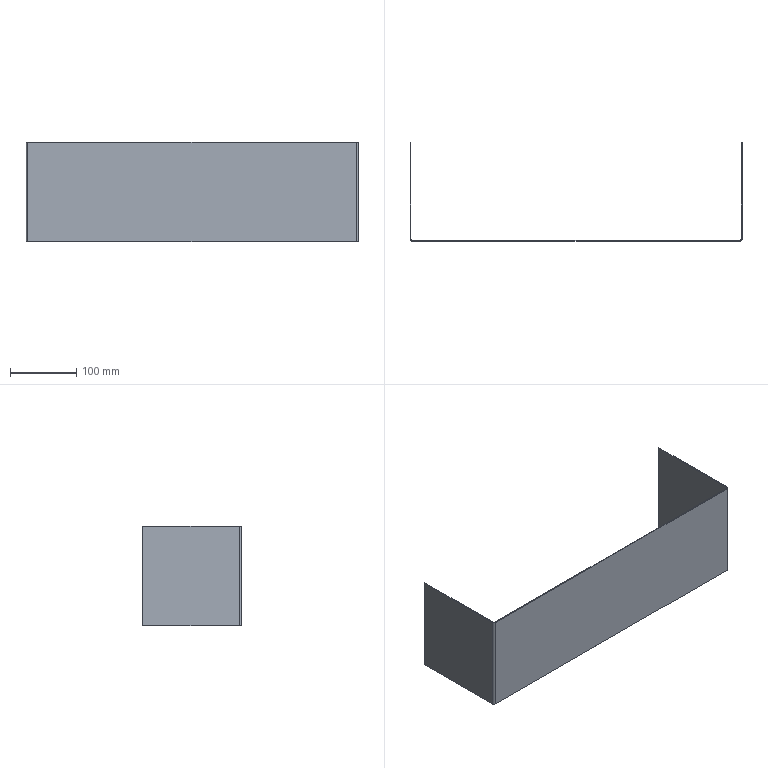Part | STEP file | 750038221 | 1 solid | 14 faces | box 500 x 148.5 x 150 mm | volume 178215 mm3 | plane 10 | cylinder 4 | commonest cylinder face diameters 3 x2 6 x2
STEP:
#1=CARTESIAN_POINT('',(-247.,0.,0.));
#2=VERTEX_POINT('',#1);
#3=CARTESIAN_POINT('',(-247.,0.,150.));
#4=VERTEX_POINT('',#3);
#5=CARTESIAN_POINT('',(-247.,0.,0.));
#6=DIRECTION('',(0.,0.,1.));
#7=VECTOR('',#6,1000.);
#8=LINE('',#5,#7);
#9=EDGE_CURVE('',#2,#4,#8,.T.);
#10=ORIENTED_EDGE('',*,*,#9,.F.);
#11=CARTESIAN_POINT('',(247.,0.,0.));
#12=VERTEX_POINT('',#11);
#13=CARTESIAN_POINT('',(250.,0.,0.));
#14=DIRECTION('',(-1.,0.,0.));
#15=VECTOR('',#14,1000.);
#16=LINE('',#13,#15);
#17=EDGE_CURVE('',#12,#2,#16,.T.);
#18=ORIENTED_EDGE('',*,*,#17,.F.);
#19=CARTESIAN_POINT('',(247.,0.,150.));
#20=VERTEX_POINT('',#19);
#21=CARTESIAN_POINT('',(247.,0.,0.));
#22=DIRECTION('',(0.,0.,-1.));
#23=VECTOR('',#22,1000.);
#24=LINE('',#21,#23);
#25=EDGE_CURVE('',#20,#12,#24,.T.);
#26=ORIENTED_EDGE('',*,*,#25,.F.);
#27=CARTESIAN_POINT('',(250.,0.,150.));
#28=DIRECTION('',(1.,0.,0.));
#29=VECTOR('',#28,1000.);
#30=LINE('',#27,#29);
#31=EDGE_CURVE('',#4,#20,#30,.T.);
#32=ORIENTED_EDGE('',*,*,#31,.F.);
#33=EDGE_LOOP('',(#10,#18,#26,#32));
#34=FACE_OUTER_BOUND('',#33,.T.);
#35=CARTESIAN_POINT('',(250.,0.,0.));
#36=DIRECTION('',(0.,1.,0.));
#37=DIRECTION('',(-1.,0.,0.));
#38=AXIS2_PLACEMENT_3D('',#35,#36,#37);
#39=PLANE('',#38);
#40=ADVANCED_FACE('',(#34),#39,.F.);
#41=CARTESIAN_POINT('',(-247.,1.5,150.));
#42=VERTEX_POINT('',#41);
#43=CARTESIAN_POINT('',(247.,1.5,150.));
#44=VERTEX_POINT('',#43);
#45=CARTESIAN_POINT('',(247.,1.5,150.));
#46=DIRECTION('',(1.,0.,0.));
#47=VECTOR('',#46,1000.);
#48=LINE('',#45,#47);
#49=EDGE_CURVE('',#42,#44,#48,.T.);
#50=ORIENTED_EDGE('',*,*,#49,.F.);
#51=CARTESIAN_POINT('',(-248.5,3.,150.));
#52=VERTEX_POINT('',#51);
#53=CARTESIAN_POINT('',(-247.,3.,150.));
#54=DIRECTION('',(0.,0.,1.));
#55=DIRECTION('',(1.,0.,0.));
#56=AXIS2_PLACEMENT_3D('',#53,#54,#55);
#57=CIRCLE('',#56,1.5);
#58=EDGE_CURVE('',#52,#42,#57,.T.);
#59=ORIENTED_EDGE('',*,*,#58,.F.);
#60=CARTESIAN_POINT('',(-248.5,148.5,150.));
#61=VERTEX_POINT('',#60);
#62=CARTESIAN_POINT('',(-248.5,3.,150.));
#63=DIRECTION('',(0.,-1.,0.));
#64=VECTOR('',#63,1000.);
#65=LINE('',#62,#64);
#66=EDGE_CURVE('',#61,#52,#65,.T.);
#67=ORIENTED_EDGE('',*,*,#66,.F.);
#68=CARTESIAN_POINT('',(-250.,148.5,150.));
#69=VERTEX_POINT('',#68);
#70=CARTESIAN_POINT('',(-250.,148.5,150.));
#71=DIRECTION('',(1.,0.,0.));
#72=VECTOR('',#71,1000.);
#73=LINE('',#70,#72);
#74=EDGE_CURVE('',#69,#61,#73,.T.);
#75=ORIENTED_EDGE('',*,*,#74,.F.);
#76=CARTESIAN_POINT('',(-250.,3.,150.));
#77=VERTEX_POINT('',#76);
#78=CARTESIAN_POINT('',(-250.,3.,150.));
#79=DIRECTION('',(0.,1.,0.));
#80=VECTOR('',#79,1000.);
#81=LINE('',#78,#80);
#82=EDGE_CURVE('',#77,#69,#81,.T.);
#83=ORIENTED_EDGE('',*,*,#82,.F.);
#84=CARTESIAN_POINT('',(-247.,3.,150.));
#85=DIRECTION('',(0.,0.,-1.));
#86=DIRECTION('',(1.,0.,0.));
#87=AXIS2_PLACEMENT_3D('',#84,#85,#86);
#88=CIRCLE('',#87,3.);
#89=EDGE_CURVE('',#4,#77,#88,.T.);
#90=ORIENTED_EDGE('',*,*,#89,.F.);
#91=ORIENTED_EDGE('',*,*,#31,.T.);
#92=CARTESIAN_POINT('',(250.,3.,150.));
#93=VERTEX_POINT('',#92);
#94=CARTESIAN_POINT('',(247.,3.,150.));
#95=DIRECTION('',(0.,0.,-1.));
#96=DIRECTION('',(1.,0.,0.));
#97=AXIS2_PLACEMENT_3D('',#94,#95,#96);
#98=CIRCLE('',#97,3.);
#99=EDGE_CURVE('',#93,#20,#98,.T.);
#100=ORIENTED_EDGE('',*,*,#99,.F.);
#101=CARTESIAN_POINT('',(250.,148.5,150.));
#102=VERTEX_POINT('',#101);
#103=CARTESIAN_POINT('',(250.,3.,150.));
#104=DIRECTION('',(0.,-1.,0.));
#105=VECTOR('',#104,1000.);
#106=LINE('',#103,#105);
#107=EDGE_CURVE('',#102,#93,#106,.T.);
#108=ORIENTED_EDGE('',*,*,#107,.F.);
#109=CARTESIAN_POINT('',(248.5,148.5,150.));
#110=VERTEX_POINT('',#109);
#111=CARTESIAN_POINT('',(250.,148.5,150.));
#112=DIRECTION('',(-1.,0.,0.));
#113=VECTOR('',#112,1000.);
#114=LINE('',#111,#113);
#115=EDGE_CURVE('',#102,#110,#114,.T.);
#116=ORIENTED_EDGE('',*,*,#115,.T.);
#117=CARTESIAN_POINT('',(248.5,3.,150.));
#118=VERTEX_POINT('',#117);
#119=CARTESIAN_POINT('',(248.5,3.,150.));
#120=DIRECTION('',(0.,1.,0.));
#121=VECTOR('',#120,1000.);
#122=LINE('',#119,#121);
#123=EDGE_CURVE('',#118,#110,#122,.T.);
#124=ORIENTED_EDGE('',*,*,#123,.F.);
#125=CARTESIAN_POINT('',(247.,3.,150.));
#126=DIRECTION('',(0.,0.,1.));
#127=DIRECTION('',(1.,0.,0.));
#128=AXIS2_PLACEMENT_3D('',#125,#126,#127);
#129=CIRCLE('',#128,1.5);
#130=EDGE_CURVE('',#44,#118,#129,.T.);
#131=ORIENTED_EDGE('',*,*,#130,.F.);
#132=EDGE_LOOP('',(#50,#59,#67,#75,#83,#90,#91,#100,#108,#116,#124,#131));
#133=FACE_OUTER_BOUND('',#132,.T.);
#134=CARTESIAN_POINT('',(247.,3.,150.));
#135=DIRECTION('',(0.,0.,-1.));
#136=DIRECTION('',(-1.,0.,0.));
#137=AXIS2_PLACEMENT_3D('',#134,#135,#136);
#138=PLANE('',#137);
#139=ADVANCED_FACE('',(#133),#138,.F.);
#140=CARTESIAN_POINT('',(-250.,3.,0.));
#141=VERTEX_POINT('',#140);
#142=CARTESIAN_POINT('',(-247.,3.,0.));
#143=DIRECTION('',(0.,0.,1.));
#144=DIRECTION('',(1.,0.,0.));
#145=AXIS2_PLACEMENT_3D('',#142,#143,#144);
#146=CIRCLE('',#145,3.);
#147=EDGE_CURVE('',#141,#2,#146,.T.);
#148=ORIENTED_EDGE('',*,*,#147,.T.);
#149=ORIENTED_EDGE('',*,*,#9,.T.);
#150=ORIENTED_EDGE('',*,*,#89,.T.);
#151=CARTESIAN_POINT('',(-250.,3.,0.));
#152=DIRECTION('',(0.,0.,-1.));
#153=VECTOR('',#152,1000.);
#154=LINE('',#151,#153);
#155=EDGE_CURVE('',#77,#141,#154,.T.);
#156=ORIENTED_EDGE('',*,*,#155,.T.);
#157=EDGE_LOOP('',(#148,#149,#150,#156));
#158=FACE_OUTER_BOUND('',#157,.T.);
#159=CARTESIAN_POINT('',(-247.,3.,0.));
#160=DIRECTION('',(0.,0.,1.));
#161=DIRECTION('',(1.,0.,0.));
#162=AXIS2_PLACEMENT_3D('',#159,#160,#161);
#163=CYLINDRICAL_SURFACE('',#162,3.);
#164=ADVANCED_FACE('',(#158),#163,.T.);
#165=CARTESIAN_POINT('',(248.5,3.,0.));
#166=VERTEX_POINT('',#165);
#167=CARTESIAN_POINT('',(248.5,148.5,0.));
#168=VERTEX_POINT('',#167);
#169=CARTESIAN_POINT('',(248.5,148.5,0.));
#170=DIRECTION('',(0.,1.,0.));
#171=VECTOR('',#170,1000.);
#172=LINE('',#169,#171);
#173=EDGE_CURVE('',#166,#168,#172,.T.);
#174=ORIENTED_EDGE('',*,*,#173,.T.);
#175=CARTESIAN_POINT('',(250.,148.5,0.));
#176=VERTEX_POINT('',#175);
#177=CARTESIAN_POINT('',(250.,148.5,0.));
#178=DIRECTION('',(1.,0.,0.));
#179=VECTOR('',#178,1000.);
#180=LINE('',#177,#179);
#181=EDGE_CURVE('',#168,#176,#180,.T.);
#182=ORIENTED_EDGE('',*,*,#181,.T.);
#183=CARTESIAN_POINT('',(250.,3.,0.));
#184=VERTEX_POINT('',#183);
#185=CARTESIAN_POINT('',(250.,148.5,0.));
#186=DIRECTION('',(0.,-1.,0.));
#187=VECTOR('',#186,1000.);
#188=LINE('',#185,#187);
#189=EDGE_CURVE('',#176,#184,#188,.T.);
#190=ORIENTED_EDGE('',*,*,#189,.T.);
#191=CARTESIAN_POINT('',(247.,3.,0.));
#192=DIRECTION('',(0.,0.,-1.));
#193=DIRECTION('',(1.,0.,0.));
#194=AXIS2_PLACEMENT_3D('',#191,#192,#193);
#195=CIRCLE('',#194,3.);
#196=EDGE_CURVE('',#184,#12,#195,.T.);
#197=ORIENTED_EDGE('',*,*,#196,.T.);
#198=ORIENTED_EDGE('',*,*,#17,.T.);
#199=ORIENTED_EDGE('',*,*,#147,.F.);
#200=CARTESIAN_POINT('',(-250.,148.5,0.));
#201=VERTEX_POINT('',#200);
#202=CARTESIAN_POINT('',(-250.,148.5,0.));
#203=DIRECTION('',(0.,1.,0.));
#204=VECTOR('',#203,1000.);
#205=LINE('',#202,#204);
#206=EDGE_CURVE('',#141,#201,#205,.T.);
#207=ORIENTED_EDGE('',*,*,#206,.T.);
#208=CARTESIAN_POINT('',(-248.5,148.5,0.));
#209=VERTEX_POINT('',#208);
#210=CARTESIAN_POINT('',(-250.,148.5,0.));
#211=DIRECTION('',(-1.,0.,0.));
#212=VECTOR('',#211,1000.);
#213=LINE('',#210,#212);
#214=EDGE_CURVE('',#209,#201,#213,.T.);
#215=ORIENTED_EDGE('',*,*,#214,.F.);
#216=CARTESIAN_POINT('',(-248.5,3.,0.));
#217=VERTEX_POINT('',#216);
#218=CARTESIAN_POINT('',(-248.5,148.5,0.));
#219=DIRECTION('',(0.,-1.,0.));
#220=VECTOR('',#219,1000.);
#221=LINE('',#218,#220);
#222=EDGE_CURVE('',#209,#217,#221,.T.);
#223=ORIENTED_EDGE('',*,*,#222,.T.);
#224=CARTESIAN_POINT('',(-247.,1.5,0.));
#225=VERTEX_POINT('',#224);
#226=CARTESIAN_POINT('',(-247.,3.,0.));
#227=DIRECTION('',(0.,0.,1.));
#228=DIRECTION('',(1.,0.,0.));
#229=AXIS2_PLACEMENT_3D('',#226,#227,#228);
#230=CIRCLE('',#229,1.5);
#231=EDGE_CURVE('',#217,#225,#230,.T.);
#232=ORIENTED_EDGE('',*,*,#231,.T.);
#233=CARTESIAN_POINT('',(247.,1.5,0.));
#234=VERTEX_POINT('',#233);
#235=CARTESIAN_POINT('',(250.,1.5,0.));
#236=DIRECTION('',(1.,0.,0.));
#237=VECTOR('',#236,1000.);
#238=LINE('',#235,#237);
#239=EDGE_CURVE('',#225,#234,#238,.T.);
#240=ORIENTED_EDGE('',*,*,#239,.T.);
#241=CARTESIAN_POINT('',(247.,3.,0.));
#242=DIRECTION('',(0.,0.,1.));
#243=DIRECTION('',(1.,0.,0.));
#244=AXIS2_PLACEMENT_3D('',#241,#242,#243);
#245=CIRCLE('',#244,1.5);
#246=EDGE_CURVE('',#234,#166,#245,.T.);
#247=ORIENTED_EDGE('',*,*,#246,.T.);
#248=EDGE_LOOP('',(#174,#182,#190,#197,#198,#199,#207,#215,#223,#232,#240,#247));
#249=FACE_OUTER_BOUND('',#248,.T.);
#250=CARTESIAN_POINT('',(250.,148.5,0.));
#251=DIRECTION('',(0.,0.,-1.));
#252=DIRECTION('',(-1.,0.,0.));
#253=AXIS2_PLACEMENT_3D('',#250,#251,#252);
#254=PLANE('',#253);
#255=ADVANCED_FACE('',(#249),#254,.T.);
#256=ORIENTED_EDGE('',*,*,#196,.F.);
#257=CARTESIAN_POINT('',(250.,3.,0.));
#258=DIRECTION('',(0.,0.,1.));
#259=VECTOR('',#258,1000.);
#260=LINE('',#257,#259);
#261=EDGE_CURVE('',#184,#93,#260,.T.);
#262=ORIENTED_EDGE('',*,*,#261,.T.);
#263=ORIENTED_EDGE('',*,*,#99,.T.);
#264=ORIENTED_EDGE('',*,*,#25,.T.);
#265=EDGE_LOOP('',(#256,#262,#263,#264));
#266=FACE_OUTER_BOUND('',#265,.T.);
#267=CARTESIAN_POINT('',(247.,3.,0.));
#268=DIRECTION('',(0.,0.,1.));
#269=DIRECTION('',(1.,0.,0.));
#270=AXIS2_PLACEMENT_3D('',#267,#268,#269);
#271=CYLINDRICAL_SURFACE('',#270,3.);
#272=ADVANCED_FACE('',(#266),#271,.T.);
#273=CARTESIAN_POINT('',(248.5,3.,0.));
#274=DIRECTION('',(0.,0.,1.));
#275=VECTOR('',#274,1000.);
#276=LINE('',#273,#275);
#277=EDGE_CURVE('',#166,#118,#276,.T.);
#278=ORIENTED_EDGE('',*,*,#277,.F.);
#279=ORIENTED_EDGE('',*,*,#246,.F.);
#280=CARTESIAN_POINT('',(247.,1.5,0.));
#281=DIRECTION('',(0.,0.,-1.));
#282=VECTOR('',#281,1000.);
#283=LINE('',#280,#282);
#284=EDGE_CURVE('',#44,#234,#283,.T.);
#285=ORIENTED_EDGE('',*,*,#284,.F.);
#286=ORIENTED_EDGE('',*,*,#130,.T.);
#287=EDGE_LOOP('',(#278,#279,#285,#286));
#288=FACE_OUTER_BOUND('',#287,.T.);
#289=CARTESIAN_POINT('',(247.,3.,0.));
#290=DIRECTION('',(0.,0.,1.));
#291=DIRECTION('',(1.,0.,0.));
#292=AXIS2_PLACEMENT_3D('',#289,#290,#291);
#293=CYLINDRICAL_SURFACE('',#292,1.5);
#294=ADVANCED_FACE('',(#288),#293,.F.);
#295=ORIENTED_EDGE('',*,*,#239,.F.);
#296=CARTESIAN_POINT('',(-247.,1.5,0.));
#297=DIRECTION('',(0.,0.,1.));
#298=VECTOR('',#297,1000.);
#299=LINE('',#296,#298);
#300=EDGE_CURVE('',#225,#42,#299,.T.);
#301=ORIENTED_EDGE('',*,*,#300,.T.);
#302=ORIENTED_EDGE('',*,*,#49,.T.);
#303=ORIENTED_EDGE('',*,*,#284,.T.);
#304=EDGE_LOOP('',(#295,#301,#302,#303));
#305=FACE_OUTER_BOUND('',#304,.T.);
#306=CARTESIAN_POINT('',(250.,1.5,0.));
#307=DIRECTION('',(0.,1.,0.));
#308=DIRECTION('',(-1.,0.,0.));
#309=AXIS2_PLACEMENT_3D('',#306,#307,#308);
#310=PLANE('',#309);
#311=ADVANCED_FACE('',(#305),#310,.T.);
#312=ORIENTED_EDGE('',*,*,#300,.F.);
#313=ORIENTED_EDGE('',*,*,#231,.F.);
#314=CARTESIAN_POINT('',(-248.5,3.,0.));
#315=DIRECTION('',(0.,0.,-1.));
#316=VECTOR('',#315,1000.);
#317=LINE('',#314,#316);
#318=EDGE_CURVE('',#52,#217,#317,.T.);
#319=ORIENTED_EDGE('',*,*,#318,.F.);
#320=ORIENTED_EDGE('',*,*,#58,.T.);
#321=EDGE_LOOP('',(#312,#313,#319,#320));
#322=FACE_OUTER_BOUND('',#321,.T.);
#323=CARTESIAN_POINT('',(-247.,3.,0.));
#324=DIRECTION('',(0.,0.,1.));
#325=DIRECTION('',(1.,0.,0.));
#326=AXIS2_PLACEMENT_3D('',#323,#324,#325);
#327=CYLINDRICAL_SURFACE('',#326,1.5);
#328=ADVANCED_FACE('',(#322),#327,.F.);
#329=ORIENTED_EDGE('',*,*,#222,.F.);
#330=CARTESIAN_POINT('',(-248.5,148.5,0.));
#331=DIRECTION('',(0.,0.,1.));
#332=VECTOR('',#331,1000.);
#333=LINE('',#330,#332);
#334=EDGE_CURVE('',#209,#61,#333,.T.);
#335=ORIENTED_EDGE('',*,*,#334,.T.);
#336=ORIENTED_EDGE('',*,*,#66,.T.);
#337=ORIENTED_EDGE('',*,*,#318,.T.);
#338=EDGE_LOOP('',(#329,#335,#336,#337));
#339=FACE_OUTER_BOUND('',#338,.T.);
#340=CARTESIAN_POINT('',(-248.5,0.,0.));
#341=DIRECTION('',(1.,0.,0.));
#342=DIRECTION('',(0.,1.,0.));
#343=AXIS2_PLACEMENT_3D('',#340,#341,#342);
#344=PLANE('',#343);
#345=ADVANCED_FACE('',(#339),#344,.T.);
#346=CARTESIAN_POINT('',(-250.,148.5,0.));
#347=DIRECTION('',(0.,0.,1.));
#348=VECTOR('',#347,1000.);
#349=LINE('',#346,#348);
#350=EDGE_CURVE('',#201,#69,#349,.T.);
#351=ORIENTED_EDGE('',*,*,#350,.F.);
#352=ORIENTED_EDGE('',*,*,#206,.F.);
#353=ORIENTED_EDGE('',*,*,#155,.F.);
#354=ORIENTED_EDGE('',*,*,#82,.T.);
#355=EDGE_LOOP('',(#351,#352,#353,#354));
#356=FACE_OUTER_BOUND('',#355,.T.);
#357=CARTESIAN_POINT('',(-250.,0.,0.));
#358=DIRECTION('',(1.,0.,0.));
#359=DIRECTION('',(0.,1.,0.));
#360=AXIS2_PLACEMENT_3D('',#357,#358,#359);
#361=PLANE('',#360);
#362=ADVANCED_FACE('',(#356),#361,.F.);
#363=ORIENTED_EDGE('',*,*,#261,.F.);
#364=ORIENTED_EDGE('',*,*,#189,.F.);
#365=CARTESIAN_POINT('',(250.,148.5,0.));
#366=DIRECTION('',(0.,0.,-1.));
#367=VECTOR('',#366,1000.);
#368=LINE('',#365,#367);
#369=EDGE_CURVE('',#102,#176,#368,.T.);
#370=ORIENTED_EDGE('',*,*,#369,.F.);
#371=ORIENTED_EDGE('',*,*,#107,.T.);
#372=EDGE_LOOP('',(#363,#364,#370,#371));
#373=FACE_OUTER_BOUND('',#372,.T.);
#374=CARTESIAN_POINT('',(250.,148.5,0.));
#375=DIRECTION('',(-1.,0.,0.));
#376=DIRECTION('',(0.,-1.,0.));
#377=AXIS2_PLACEMENT_3D('',#374,#375,#376);
#378=PLANE('',#377);
#379=ADVANCED_FACE('',(#373),#378,.F.);
#380=ORIENTED_EDGE('',*,*,#173,.F.);
#381=ORIENTED_EDGE('',*,*,#277,.T.);
#382=ORIENTED_EDGE('',*,*,#123,.T.);
#383=CARTESIAN_POINT('',(248.5,148.5,0.));
#384=DIRECTION('',(0.,0.,-1.));
#385=VECTOR('',#384,1000.);
#386=LINE('',#383,#385);
#387=EDGE_CURVE('',#110,#168,#386,.T.);
#388=ORIENTED_EDGE('',*,*,#387,.T.);
#389=EDGE_LOOP('',(#380,#381,#382,#388));
#390=FACE_OUTER_BOUND('',#389,.T.);
#391=CARTESIAN_POINT('',(248.5,148.5,0.));
#392=DIRECTION('',(-1.,0.,0.));
#393=DIRECTION('',(0.,-1.,0.));
#394=AXIS2_PLACEMENT_3D('',#391,#392,#393);
#395=PLANE('',#394);
#396=ADVANCED_FACE('',(#390),#395,.T.);
#397=ORIENTED_EDGE('',*,*,#214,.T.);
#398=ORIENTED_EDGE('',*,*,#350,.T.);
#399=ORIENTED_EDGE('',*,*,#74,.T.);
#400=ORIENTED_EDGE('',*,*,#334,.F.);
#401=EDGE_LOOP('',(#397,#398,#399,#400));
#402=FACE_OUTER_BOUND('',#401,.T.);
#403=CARTESIAN_POINT('',(-250.,148.5,0.));
#404=DIRECTION('',(0.,1.,0.));
#405=DIRECTION('',(-1.,0.,0.));
#406=AXIS2_PLACEMENT_3D('',#403,#404,#405);
#407=PLANE('',#406);
#408=ADVANCED_FACE('',(#402),#407,.T.);
#409=ORIENTED_EDGE('',*,*,#387,.F.);
#410=ORIENTED_EDGE('',*,*,#115,.F.);
#411=ORIENTED_EDGE('',*,*,#369,.T.);
#412=ORIENTED_EDGE('',*,*,#181,.F.);
#413=EDGE_LOOP('',(#409,#410,#411,#412));
#414=FACE_OUTER_BOUND('',#413,.T.);
#415=CARTESIAN_POINT('',(250.,148.5,0.));
#416=DIRECTION('',(0.,-1.,0.));
#417=DIRECTION('',(1.,0.,0.));
#418=AXIS2_PLACEMENT_3D('',#415,#416,#417);
#419=PLANE('',#418);
#420=ADVANCED_FACE('',(#414),#419,.F.);
#421=CLOSED_SHELL('',(#40,#139,#164,#255,#272,#294,#311,#328,#345,#362,#379,#396,#408,#420));
#422=MANIFOLD_SOLID_BREP('',#421);
#423=CARTESIAN_POINT('',(0.,0.,0.));
#424=DIRECTION('',(0.,0.,1.));
#425=DIRECTION('',(1.,0.,0.));
#426=AXIS2_PLACEMENT_3D('',#423,#424,#425);
#427=(LENGTH_UNIT()NAMED_UNIT(*)SI_UNIT(.MILLI.,.METRE.));
#428=UNCERTAINTY_MEASURE_WITH_UNIT(LENGTH_MEASURE(0.00001),#427,'','');
#429=(NAMED_UNIT(*)PLANE_ANGLE_UNIT()SI_UNIT($,.RADIAN.));
#430=(NAMED_UNIT(*)SI_UNIT($,.STERADIAN.)SOLID_ANGLE_UNIT());
#431=(GEOMETRIC_REPRESENTATION_CONTEXT(3)GLOBAL_UNCERTAINTY_ASSIGNED_CONTEXT((#428))GLOBAL_UNIT_ASSIGNED_CONTEXT((#427,#429,#430))REPRESENTATION_CONTEXT('',''));
#432=ADVANCED_BREP_SHAPE_REPRESENTATION('',(#422,#426),#431);